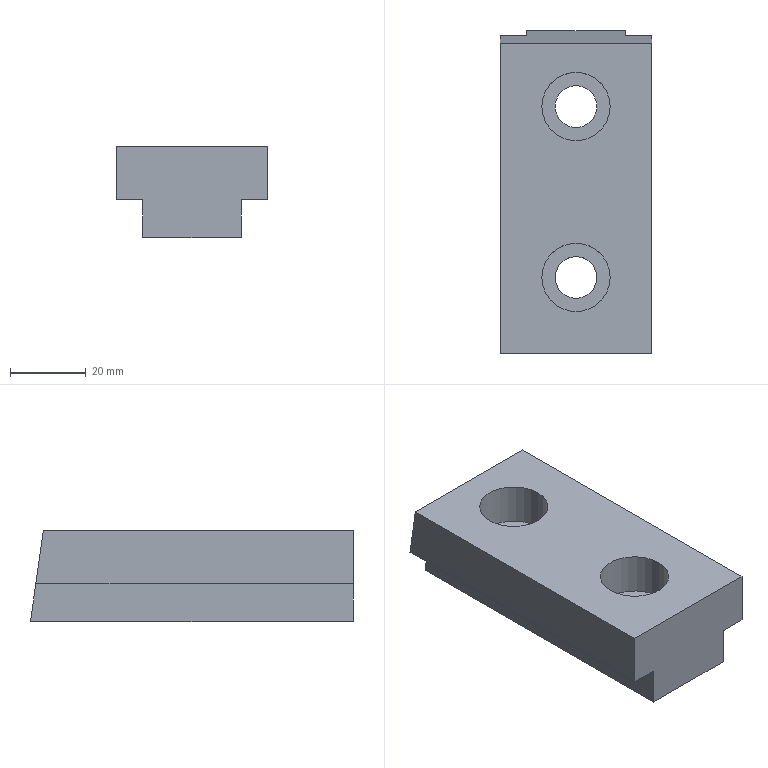Part | STEP file | solid 246 | 1 solid | 16 faces | box 40 x 85.054 x 24 mm | volume 60155 mm3 | plane 11 | cylinder 4 | spline 1 | commonest cylinder face diameters 11 x2 18 x2